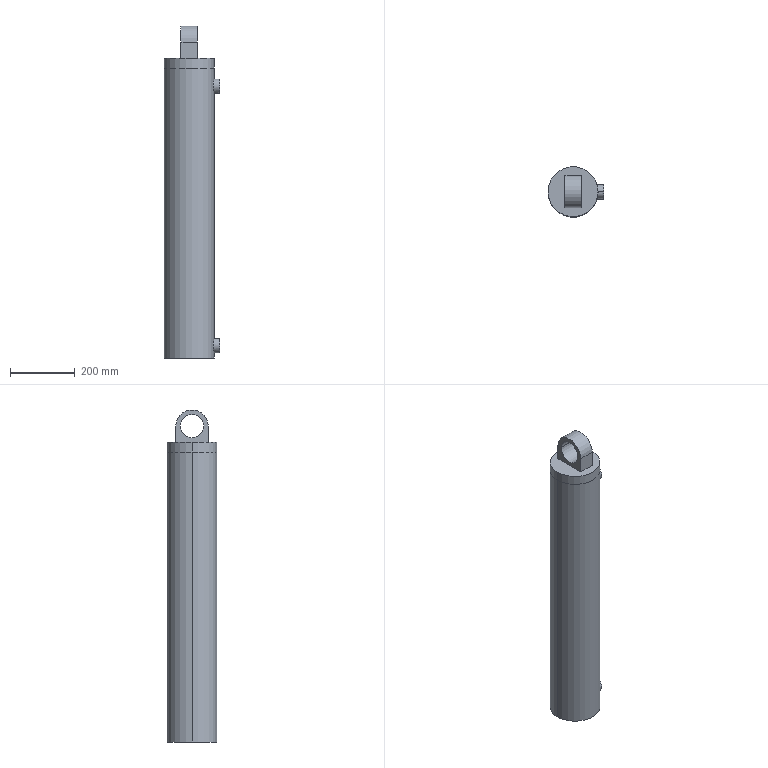Part | SolidWorks | features BaseBody 2, ICE 1 | 2 solids | 41 faces | box 172 x 154 x 1025 mm | volume 9175739 mm3 | cylinder 26 | plane 15 | commonest cylinder face diameters 43.629 x9 10 x8 154 x4 72 x2 110 x2 100 x1